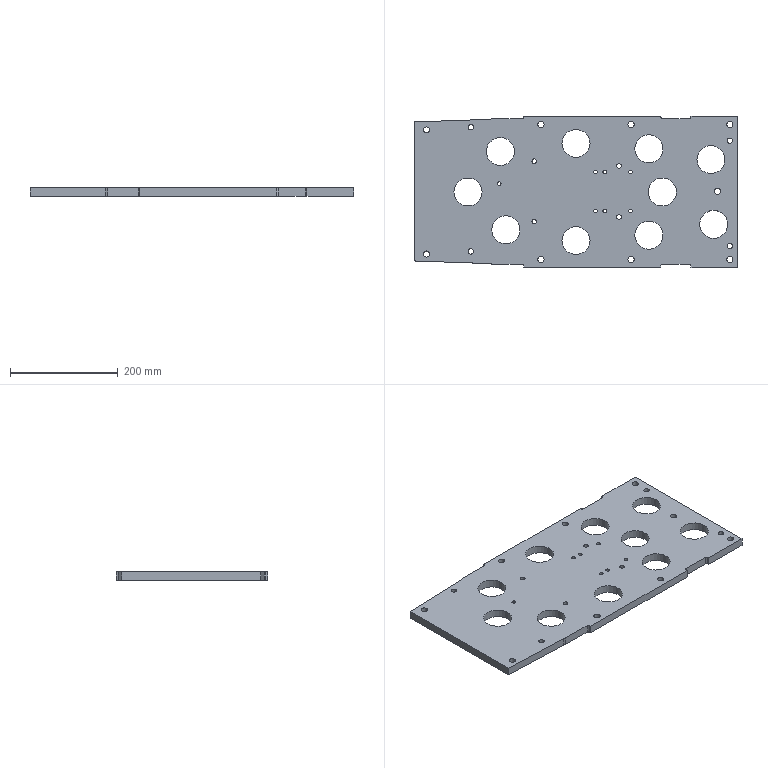Part | NX | features UB-10 2 | 1 solid | 73 faces | box 600 x 280 x 15 mm | volume 2120645 mm3 | cylinder 42 | plane 20 | cone 11 | commonest cylinder face diameters 52.004 x10 11.507 x9 6 x6 6.8 x6 8.5 x4 10 x4